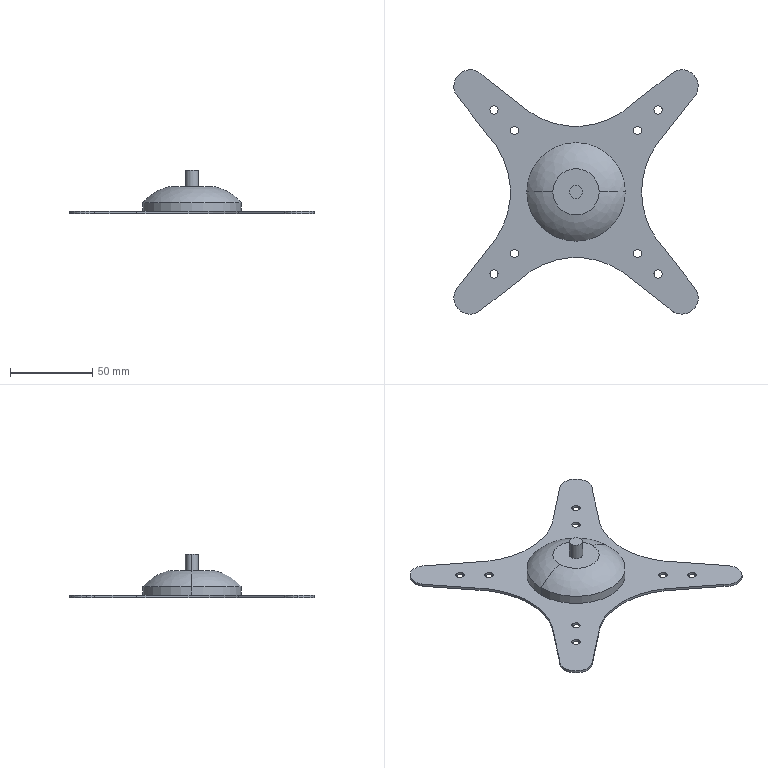Part | SolidWorks | features ICE 3, Extrusion 1, RefAxis 1, RevCut 1 | 1 solid | 45 faces | box 148.985 x 148.985 x 26.5 mm | volume 50583 mm3 | cylinder 31 | plane 12 | spline 2 | commonest cylinder face diameters 5 x16 20 x6 100 x5 8 x2 60 x2
STEP:
#1=CARTESIAN_POINT('',(-30.,0.,6.799));
#2=VERTEX_POINT('',#1);
#3=CARTESIAN_POINT('',(30.,0.,6.799));
#4=VERTEX_POINT('',#3);
#5=CARTESIAN_POINT('',(0.,0.,6.799));
#6=DIRECTION('',(0.,0.,-1.));
#7=DIRECTION('',(-1.,0.,0.));
#8=AXIS2_PLACEMENT_3D('',#5,#6,#7);
#9=CIRCLE('',#8,30.);
#10=EDGE_CURVE('',#2,#4,#9,.T.);
#11=ORIENTED_EDGE('',*,*,#10,.F.);
#12=CARTESIAN_POINT('',(-14.118,0.,16.5));
#13=VERTEX_POINT('',#12);
#14=CARTESIAN_POINT('',(-30.,0.,6.799));
#15=CARTESIAN_POINT('',(-23.65,0.,14.105));
#16=CARTESIAN_POINT('',(-14.118,0.,16.5));
#17=B_SPLINE_CURVE_WITH_KNOTS('',2,(#14,#15,#16),.UNSPECIFIED.,.F.,.F.,(3,3),(0.,1.),.UNSPECIFIED.);
#18=EDGE_CURVE('',#2,#13,#17,.T.);
#19=ORIENTED_EDGE('',*,*,#18,.T.);
#20=CARTESIAN_POINT('',(14.118,0.,16.5));
#21=VERTEX_POINT('',#20);
#22=CARTESIAN_POINT('',(0.,0.,16.5));
#23=DIRECTION('',(0.,0.,-1.));
#24=DIRECTION('',(-1.,0.,0.));
#25=AXIS2_PLACEMENT_3D('',#22,#23,#24);
#26=CIRCLE('',#25,14.118);
#27=EDGE_CURVE('',#13,#21,#26,.T.);
#28=ORIENTED_EDGE('',*,*,#27,.T.);
#29=CARTESIAN_POINT('',(30.,0.,6.799));
#30=CARTESIAN_POINT('',(23.65,0.,14.105));
#31=CARTESIAN_POINT('',(14.118,0.,16.5));
#32=B_SPLINE_CURVE_WITH_KNOTS('',2,(#29,#30,#31),.UNSPECIFIED.,.F.,.F.,(3,3),(0.,1.),.UNSPECIFIED.);
#33=EDGE_CURVE('',#4,#21,#32,.T.);
#34=ORIENTED_EDGE('',*,*,#33,.F.);
#35=EDGE_LOOP('',(#11,#19,#28,#34));
#36=FACE_OUTER_BOUND('',#35,.T.);
#37=CARTESIAN_POINT('',(-30.,0.,6.799));
#38=CARTESIAN_POINT('',(-30.,60.,6.799));
#39=CARTESIAN_POINT('',(30.,60.,6.799));
#40=CARTESIAN_POINT('',(30.,0.,6.799));
#41=CARTESIAN_POINT('',(-23.65,0.,14.105));
#42=CARTESIAN_POINT('',(-23.65,47.299,14.105));
#43=CARTESIAN_POINT('',(23.65,47.299,14.105));
#44=CARTESIAN_POINT('',(23.65,0.,14.105));
#45=CARTESIAN_POINT('',(-14.118,0.,16.5));
#46=CARTESIAN_POINT('',(-14.118,28.237,16.5));
#47=CARTESIAN_POINT('',(14.118,28.237,16.5));
#48=CARTESIAN_POINT('',(14.118,0.,16.5));
#49=(BOUNDED_SURFACE()B_SPLINE_SURFACE(2,3,((#37,#38,#39,#40),(#41,#42,#43,#44),(#45,#46,#47,#48)),.UNSPECIFIED.,.F.,.F.,.F.)B_SPLINE_SURFACE_WITH_KNOTS((3,3),(4,4),(0.,1.),(0.,1.),.UNSPECIFIED.)GEOMETRIC_REPRESENTATION_ITEM()RATIONAL_B_SPLINE_SURFACE(((1.,0.3333,0.3333,1.),(1.,0.3333,0.3333,1.),(1.,0.3333,0.3333,1.)))REPRESENTATION_ITEM('')SURFACE());
#50=ADVANCED_FACE('',(#36),#49,.T.);
#51=CARTESIAN_POINT('',(4.,0.,26.5));
#52=VERTEX_POINT('',#51);
#53=CARTESIAN_POINT('',(-4.,0.,26.5));
#54=VERTEX_POINT('',#53);
#55=CARTESIAN_POINT('',(0.,0.,26.5));
#56=DIRECTION('',(0.,0.,1.));
#57=DIRECTION('',(1.,0.,0.));
#58=AXIS2_PLACEMENT_3D('',#55,#56,#57);
#59=CIRCLE('',#58,4.);
#60=EDGE_CURVE('',#52,#54,#59,.T.);
#61=ORIENTED_EDGE('',*,*,#60,.F.);
#62=CARTESIAN_POINT('',(4.,0.,16.5));
#63=VERTEX_POINT('',#62);
#64=CARTESIAN_POINT('',(4.,0.,26.5));
#65=DIRECTION('',(0.,0.,-1.));
#66=VECTOR('',#65,1000.);
#67=LINE('',#64,#66);
#68=EDGE_CURVE('',#52,#63,#67,.T.);
#69=ORIENTED_EDGE('',*,*,#68,.T.);
#70=CARTESIAN_POINT('',(-4.,0.,16.5));
#71=VERTEX_POINT('',#70);
#72=CARTESIAN_POINT('',(0.,0.,16.5));
#73=DIRECTION('',(0.,0.,1.));
#74=DIRECTION('',(1.,0.,0.));
#75=AXIS2_PLACEMENT_3D('',#72,#73,#74);
#76=CIRCLE('',#75,4.);
#77=EDGE_CURVE('',#63,#71,#76,.T.);
#78=ORIENTED_EDGE('',*,*,#77,.T.);
#79=CARTESIAN_POINT('',(-4.,0.,26.5));
#80=DIRECTION('',(0.,0.,-1.));
#81=VECTOR('',#80,1000.);
#82=LINE('',#79,#81);
#83=EDGE_CURVE('',#54,#71,#82,.T.);
#84=ORIENTED_EDGE('',*,*,#83,.F.);
#85=EDGE_LOOP('',(#61,#69,#78,#84));
#86=FACE_OUTER_BOUND('',#85,.T.);
#87=CARTESIAN_POINT('',(0.,0.,26.5));
#88=DIRECTION('',(0.,0.,-1.));
#89=DIRECTION('',(-1.,0.,0.));
#90=AXIS2_PLACEMENT_3D('',#87,#88,#89);
#91=CYLINDRICAL_SURFACE('',#90,4.);
#92=ADVANCED_FACE('',(#86),#91,.T.);
#93=CARTESIAN_POINT('',(-40.,-37.5,0.));
#94=VERTEX_POINT('',#93);
#95=CARTESIAN_POINT('',(-35.,-37.5,0.));
#96=VERTEX_POINT('',#95);
#97=CARTESIAN_POINT('',(-37.5,-37.5,0.));
#98=DIRECTION('',(0.,0.,1.));
#99=DIRECTION('',(1.,0.,0.));
#100=AXIS2_PLACEMENT_3D('',#97,#98,#99);
#101=CIRCLE('',#100,2.5);
#102=EDGE_CURVE('',#94,#96,#101,.T.);
#103=ORIENTED_EDGE('',*,*,#102,.F.);
#104=CARTESIAN_POINT('',(-40.,-37.5,1.5));
#105=VERTEX_POINT('',#104);
#106=CARTESIAN_POINT('',(-40.,-37.5,0.));
#107=DIRECTION('',(0.,0.,1.));
#108=VECTOR('',#107,1000.);
#109=LINE('',#106,#108);
#110=EDGE_CURVE('',#94,#105,#109,.T.);
#111=ORIENTED_EDGE('',*,*,#110,.T.);
#112=CARTESIAN_POINT('',(-35.,-37.5,1.5));
#113=VERTEX_POINT('',#112);
#114=CARTESIAN_POINT('',(-37.5,-37.5,1.5));
#115=DIRECTION('',(0.,0.,1.));
#116=DIRECTION('',(1.,0.,0.));
#117=AXIS2_PLACEMENT_3D('',#114,#115,#116);
#118=CIRCLE('',#117,2.5);
#119=EDGE_CURVE('',#105,#113,#118,.T.);
#120=ORIENTED_EDGE('',*,*,#119,.T.);
#121=CARTESIAN_POINT('',(-35.,-37.5,0.));
#122=DIRECTION('',(0.,0.,1.));
#123=VECTOR('',#122,1000.);
#124=LINE('',#121,#123);
#125=EDGE_CURVE('',#96,#113,#124,.T.);
#126=ORIENTED_EDGE('',*,*,#125,.F.);
#127=EDGE_LOOP('',(#103,#111,#120,#126));
#128=FACE_OUTER_BOUND('',#127,.T.);
#129=CARTESIAN_POINT('',(-37.5,-37.5,0.));
#130=DIRECTION('',(0.,0.,1.));
#131=DIRECTION('',(1.,0.,0.));
#132=AXIS2_PLACEMENT_3D('',#129,#130,#131);
#133=CYLINDRICAL_SURFACE('',#132,2.5);
#134=ADVANCED_FACE('',(#128),#133,.F.);
#135=CARTESIAN_POINT('',(-52.5,-50.,0.));
#136=VERTEX_POINT('',#135);
#137=CARTESIAN_POINT('',(-47.5,-50.,0.));
#138=VERTEX_POINT('',#137);
#139=CARTESIAN_POINT('',(-50.,-50.,0.));
#140=DIRECTION('',(0.,0.,1.));
#141=DIRECTION('',(1.,0.,0.));
#142=AXIS2_PLACEMENT_3D('',#139,#140,#141);
#143=CIRCLE('',#142,2.5);
#144=EDGE_CURVE('',#136,#138,#143,.T.);
#145=ORIENTED_EDGE('',*,*,#144,.F.);
#146=CARTESIAN_POINT('',(-52.5,-50.,1.5));
#147=VERTEX_POINT('',#146);
#148=CARTESIAN_POINT('',(-52.5,-50.,0.));
#149=DIRECTION('',(0.,0.,1.));
#150=VECTOR('',#149,1000.);
#151=LINE('',#148,#150);
#152=EDGE_CURVE('',#136,#147,#151,.T.);
#153=ORIENTED_EDGE('',*,*,#152,.T.);
#154=CARTESIAN_POINT('',(-47.5,-50.,1.5));
#155=VERTEX_POINT('',#154);
#156=CARTESIAN_POINT('',(-50.,-50.,1.5));
#157=DIRECTION('',(0.,0.,1.));
#158=DIRECTION('',(1.,0.,0.));
#159=AXIS2_PLACEMENT_3D('',#156,#157,#158);
#160=CIRCLE('',#159,2.5);
#161=EDGE_CURVE('',#147,#155,#160,.T.);
#162=ORIENTED_EDGE('',*,*,#161,.T.);
#163=CARTESIAN_POINT('',(-47.5,-50.,0.));
#164=DIRECTION('',(0.,0.,1.));
#165=VECTOR('',#164,1000.);
#166=LINE('',#163,#165);
#167=EDGE_CURVE('',#138,#155,#166,.T.);
#168=ORIENTED_EDGE('',*,*,#167,.F.);
#169=EDGE_LOOP('',(#145,#153,#162,#168));
#170=FACE_OUTER_BOUND('',#169,.T.);
#171=CARTESIAN_POINT('',(-50.,-50.,0.));
#172=DIRECTION('',(0.,0.,1.));
#173=DIRECTION('',(1.,0.,0.));
#174=AXIS2_PLACEMENT_3D('',#171,#172,#173);
#175=CYLINDRICAL_SURFACE('',#174,2.5);
#176=ADVANCED_FACE('',(#170),#175,.F.);
#177=CARTESIAN_POINT('',(35.,-37.5,0.));
#178=VERTEX_POINT('',#177);
#179=CARTESIAN_POINT('',(40.,-37.5,0.));
#180=VERTEX_POINT('',#179);
#181=CARTESIAN_POINT('',(37.5,-37.5,0.));
#182=DIRECTION('',(0.,0.,1.));
#183=DIRECTION('',(1.,0.,0.));
#184=AXIS2_PLACEMENT_3D('',#181,#182,#183);
#185=CIRCLE('',#184,2.5);
#186=EDGE_CURVE('',#178,#180,#185,.T.);
#187=ORIENTED_EDGE('',*,*,#186,.F.);
#188=CARTESIAN_POINT('',(35.,-37.5,1.5));
#189=VERTEX_POINT('',#188);
#190=CARTESIAN_POINT('',(35.,-37.5,0.));
#191=DIRECTION('',(0.,0.,1.));
#192=VECTOR('',#191,1000.);
#193=LINE('',#190,#192);
#194=EDGE_CURVE('',#178,#189,#193,.T.);
#195=ORIENTED_EDGE('',*,*,#194,.T.);
#196=CARTESIAN_POINT('',(40.,-37.5,1.5));
#197=VERTEX_POINT('',#196);
#198=CARTESIAN_POINT('',(37.5,-37.5,1.5));
#199=DIRECTION('',(0.,0.,1.));
#200=DIRECTION('',(1.,0.,0.));
#201=AXIS2_PLACEMENT_3D('',#198,#199,#200);
#202=CIRCLE('',#201,2.5);
#203=EDGE_CURVE('',#189,#197,#202,.T.);
#204=ORIENTED_EDGE('',*,*,#203,.T.);
#205=CARTESIAN_POINT('',(40.,-37.5,0.));
#206=DIRECTION('',(0.,0.,1.));
#207=VECTOR('',#206,1000.);
#208=LINE('',#205,#207);
#209=EDGE_CURVE('',#180,#197,#208,.T.);
#210=ORIENTED_EDGE('',*,*,#209,.F.);
#211=EDGE_LOOP('',(#187,#195,#204,#210));
#212=FACE_OUTER_BOUND('',#211,.T.);
#213=CARTESIAN_POINT('',(37.5,-37.5,0.));
#214=DIRECTION('',(0.,0.,1.));
#215=DIRECTION('',(1.,0.,0.));
#216=AXIS2_PLACEMENT_3D('',#213,#214,#215);
#217=CYLINDRICAL_SURFACE('',#216,2.5);
#218=ADVANCED_FACE('',(#212),#217,.F.);
#219=CARTESIAN_POINT('',(47.5,-50.,0.));
#220=VERTEX_POINT('',#219);
#221=CARTESIAN_POINT('',(52.5,-50.,0.));
#222=VERTEX_POINT('',#221);
#223=CARTESIAN_POINT('',(50.,-50.,0.));
#224=DIRECTION('',(0.,0.,1.));
#225=DIRECTION('',(1.,0.,0.));
#226=AXIS2_PLACEMENT_3D('',#223,#224,#225);
#227=CIRCLE('',#226,2.5);
#228=EDGE_CURVE('',#220,#222,#227,.T.);
#229=ORIENTED_EDGE('',*,*,#228,.F.);
#230=CARTESIAN_POINT('',(47.5,-50.,1.5));
#231=VERTEX_POINT('',#230);
#232=CARTESIAN_POINT('',(47.5,-50.,0.));
#233=DIRECTION('',(0.,0.,1.));
#234=VECTOR('',#233,1000.);
#235=LINE('',#232,#234);
#236=EDGE_CURVE('',#220,#231,#235,.T.);
#237=ORIENTED_EDGE('',*,*,#236,.T.);
#238=CARTESIAN_POINT('',(52.5,-50.,1.5));
#239=VERTEX_POINT('',#238);
#240=CARTESIAN_POINT('',(50.,-50.,1.5));
#241=DIRECTION('',(0.,0.,1.));
#242=DIRECTION('',(1.,0.,0.));
#243=AXIS2_PLACEMENT_3D('',#240,#241,#242);
#244=CIRCLE('',#243,2.5);
#245=EDGE_CURVE('',#231,#239,#244,.T.);
#246=ORIENTED_EDGE('',*,*,#245,.T.);
#247=CARTESIAN_POINT('',(52.5,-50.,0.));
#248=DIRECTION('',(0.,0.,1.));
#249=VECTOR('',#248,1000.);
#250=LINE('',#247,#249);
#251=EDGE_CURVE('',#222,#239,#250,.T.);
#252=ORIENTED_EDGE('',*,*,#251,.F.);
#253=EDGE_LOOP('',(#229,#237,#246,#252));
#254=FACE_OUTER_BOUND('',#253,.T.);
#255=CARTESIAN_POINT('',(50.,-50.,0.));
#256=DIRECTION('',(0.,0.,1.));
#257=DIRECTION('',(1.,0.,0.));
#258=AXIS2_PLACEMENT_3D('',#255,#256,#257);
#259=CYLINDRICAL_SURFACE('',#258,2.5);
#260=ADVANCED_FACE('',(#254),#259,.F.);
#261=CARTESIAN_POINT('',(35.,37.5,0.));
#262=VERTEX_POINT('',#261);
#263=CARTESIAN_POINT('',(40.,37.5,0.));
#264=VERTEX_POINT('',#263);
#265=CARTESIAN_POINT('',(37.5,37.5,0.));
#266=DIRECTION('',(0.,0.,1.));
#267=DIRECTION('',(1.,0.,0.));
#268=AXIS2_PLACEMENT_3D('',#265,#266,#267);
#269=CIRCLE('',#268,2.5);
#270=EDGE_CURVE('',#262,#264,#269,.T.);
#271=ORIENTED_EDGE('',*,*,#270,.F.);
#272=CARTESIAN_POINT('',(35.,37.5,1.5));
#273=VERTEX_POINT('',#272);
#274=CARTESIAN_POINT('',(35.,37.5,0.));
#275=DIRECTION('',(0.,0.,1.));
#276=VECTOR('',#275,1000.);
#277=LINE('',#274,#276);
#278=EDGE_CURVE('',#262,#273,#277,.T.);
#279=ORIENTED_EDGE('',*,*,#278,.T.);
#280=CARTESIAN_POINT('',(40.,37.5,1.5));
#281=VERTEX_POINT('',#280);
#282=CARTESIAN_POINT('',(37.5,37.5,1.5));
#283=DIRECTION('',(0.,0.,1.));
#284=DIRECTION('',(1.,0.,0.));
#285=AXIS2_PLACEMENT_3D('',#282,#283,#284);
#286=CIRCLE('',#285,2.5);
#287=EDGE_CURVE('',#273,#281,#286,.T.);
#288=ORIENTED_EDGE('',*,*,#287,.T.);
#289=CARTESIAN_POINT('',(40.,37.5,0.));
#290=DIRECTION('',(0.,0.,1.));
#291=VECTOR('',#290,1000.);
#292=LINE('',#289,#291);
#293=EDGE_CURVE('',#264,#281,#292,.T.);
#294=ORIENTED_EDGE('',*,*,#293,.F.);
#295=EDGE_LOOP('',(#271,#279,#288,#294));
#296=FACE_OUTER_BOUND('',#295,.T.);
#297=CARTESIAN_POINT('',(37.5,37.5,0.));
#298=DIRECTION('',(0.,0.,1.));
#299=DIRECTION('',(1.,0.,0.));
#300=AXIS2_PLACEMENT_3D('',#297,#298,#299);
#301=CYLINDRICAL_SURFACE('',#300,2.5);
#302=ADVANCED_FACE('',(#296),#301,.F.);
#303=CARTESIAN_POINT('',(47.5,50.,0.));
#304=VERTEX_POINT('',#303);
#305=CARTESIAN_POINT('',(52.5,50.,0.));
#306=VERTEX_POINT('',#305);
#307=CARTESIAN_POINT('',(50.,50.,0.));
#308=DIRECTION('',(0.,0.,1.));
#309=DIRECTION('',(1.,0.,0.));
#310=AXIS2_PLACEMENT_3D('',#307,#308,#309);
#311=CIRCLE('',#310,2.5);
#312=EDGE_CURVE('',#304,#306,#311,.T.);
#313=ORIENTED_EDGE('',*,*,#312,.F.);
#314=CARTESIAN_POINT('',(47.5,50.,1.5));
#315=VERTEX_POINT('',#314);
#316=CARTESIAN_POINT('',(47.5,50.,0.));
#317=DIRECTION('',(0.,0.,1.));
#318=VECTOR('',#317,1000.);
#319=LINE('',#316,#318);
#320=EDGE_CURVE('',#304,#315,#319,.T.);
#321=ORIENTED_EDGE('',*,*,#320,.T.);
#322=CARTESIAN_POINT('',(52.5,50.,1.5));
#323=VERTEX_POINT('',#322);
#324=CARTESIAN_POINT('',(50.,50.,1.5));
#325=DIRECTION('',(0.,0.,1.));
#326=DIRECTION('',(1.,0.,0.));
#327=AXIS2_PLACEMENT_3D('',#324,#325,#326);
#328=CIRCLE('',#327,2.5);
#329=EDGE_CURVE('',#315,#323,#328,.T.);
#330=ORIENTED_EDGE('',*,*,#329,.T.);
#331=CARTESIAN_POINT('',(52.5,50.,0.));
#332=DIRECTION('',(0.,0.,1.));
#333=VECTOR('',#332,1000.);
#334=LINE('',#331,#333);
#335=EDGE_CURVE('',#306,#323,#334,.T.);
#336=ORIENTED_EDGE('',*,*,#335,.F.);
#337=EDGE_LOOP('',(#313,#321,#330,#336));
#338=FACE_OUTER_BOUND('',#337,.T.);
#339=CARTESIAN_POINT('',(50.,50.,0.));
#340=DIRECTION('',(0.,0.,1.));
#341=DIRECTION('',(1.,0.,0.));
#342=AXIS2_PLACEMENT_3D('',#339,#340,#341);
#343=CYLINDRICAL_SURFACE('',#342,2.5);
#344=ADVANCED_FACE('',(#338),#343,.F.);
#345=CARTESIAN_POINT('',(-40.,37.5,0.));
#346=VERTEX_POINT('',#345);
#347=CARTESIAN_POINT('',(-35.,37.5,0.));
#348=VERTEX_POINT('',#347);
#349=CARTESIAN_POINT('',(-37.5,37.5,0.));
#350=DIRECTION('',(0.,0.,1.));
#351=DIRECTION('',(1.,0.,0.));
#352=AXIS2_PLACEMENT_3D('',#349,#350,#351);
#353=CIRCLE('',#352,2.5);
#354=EDGE_CURVE('',#346,#348,#353,.T.);
#355=ORIENTED_EDGE('',*,*,#354,.F.);
#356=CARTESIAN_POINT('',(-40.,37.5,1.5));
#357=VERTEX_POINT('',#356);
#358=CARTESIAN_POINT('',(-40.,37.5,0.));
#359=DIRECTION('',(0.,0.,1.));
#360=VECTOR('',#359,1000.);
#361=LINE('',#358,#360);
#362=EDGE_CURVE('',#346,#357,#361,.T.);
#363=ORIENTED_EDGE('',*,*,#362,.T.);
#364=CARTESIAN_POINT('',(-35.,37.5,1.5));
#365=VERTEX_POINT('',#364);
#366=CARTESIAN_POINT('',(-37.5,37.5,1.5));
#367=DIRECTION('',(0.,0.,1.));
#368=DIRECTION('',(1.,0.,0.));
#369=AXIS2_PLACEMENT_3D('',#366,#367,#368);
#370=CIRCLE('',#369,2.5);
#371=EDGE_CURVE('',#357,#365,#370,.T.);
#372=ORIENTED_EDGE('',*,*,#371,.T.);
#373=CARTESIAN_POINT('',(-35.,37.5,0.));
#374=DIRECTION('',(0.,0.,1.));
#375=VECTOR('',#374,1000.);
#376=LINE('',#373,#375);
#377=EDGE_CURVE('',#348,#365,#376,.T.);
#378=ORIENTED_EDGE('',*,*,#377,.F.);
#379=EDGE_LOOP('',(#355,#363,#372,#378));
#380=FACE_OUTER_BOUND('',#379,.T.);
#381=CARTESIAN_POINT('',(-37.5,37.5,0.));
#382=DIRECTION('',(0.,0.,1.));
#383=DIRECTION('',(1.,0.,0.));
#384=AXIS2_PLACEMENT_3D('',#381,#382,#383);
#385=CYLINDRICAL_SURFACE('',#384,2.5);
#386=ADVANCED_FACE('',(#380),#385,.F.);
#387=CARTESIAN_POINT('',(-52.5,50.,0.));
#388=VERTEX_POINT('',#387);
#389=CARTESIAN_POINT('',(-47.5,50.,0.));
#390=VERTEX_POINT('',#389);
#391=CARTESIAN_POINT('',(-50.,50.,0.));
#392=DIRECTION('',(0.,0.,1.));
#393=DIRECTION('',(1.,0.,0.));
#394=AXIS2_PLACEMENT_3D('',#391,#392,#393);
#395=CIRCLE('',#394,2.5);
#396=EDGE_CURVE('',#388,#390,#395,.T.);
#397=ORIENTED_EDGE('',*,*,#396,.F.);
#398=CARTESIAN_POINT('',(-52.5,50.,1.5));
#399=VERTEX_POINT('',#398);
#400=CARTESIAN_POINT('',(-52.5,50.,0.));
#401=DIRECTION('',(0.,0.,1.));
#402=VECTOR('',#401,1000.);
#403=LINE('',#400,#402);
#404=EDGE_CURVE('',#388,#399,#403,.T.);
#405=ORIENTED_EDGE('',*,*,#404,.T.);
#406=CARTESIAN_POINT('',(-47.5,50.,1.5));
#407=VERTEX_POINT('',#406);
#408=CARTESIAN_POINT('',(-50.,50.,1.5));
#409=DIRECTION('',(0.,0.,1.));
#410=DIRECTION('',(1.,0.,0.));
#411=AXIS2_PLACEMENT_3D('',#408,#409,#410);
#412=CIRCLE('',#411,2.5);
#413=EDGE_CURVE('',#399,#407,#412,.T.);
#414=ORIENTED_EDGE('',*,*,#413,.T.);
#415=CARTESIAN_POINT('',(-47.5,50.,0.));
#416=DIRECTION('',(0.,0.,1.));
#417=VECTOR('',#416,1000.);
#418=LINE('',#415,#417);
#419=EDGE_CURVE('',#390,#407,#418,.T.);
#420=ORIENTED_EDGE('',*,*,#419,.F.);
#421=EDGE_LOOP('',(#397,#405,#414,#420));
#422=FACE_OUTER_BOUND('',#421,.T.);
#423=CARTESIAN_POINT('',(-50.,50.,0.));
#424=DIRECTION('',(0.,0.,1.));
#425=DIRECTION('',(1.,0.,0.));
#426=AXIS2_PLACEMENT_3D('',#423,#424,#425);
#427=CYLINDRICAL_SURFACE('',#426,2.5);
#428=ADVANCED_FACE('',(#422),#427,.F.);
#429=CARTESIAN_POINT('',(-74.493,64.493,1.5));
#430=VERTEX_POINT('',#429);
#431=CARTESIAN_POINT('',(-72.99,59.22,1.5));
#432=VERTEX_POINT('',#431);
#433=CARTESIAN_POINT('',(-64.493,64.493,1.5));
#434=DIRECTION('',(0.,0.,1.));
#435=DIRECTION('',(1.,0.,0.));
#436=AXIS2_PLACEMENT_3D('',#433,#434,#435);
#437=CIRCLE('',#436,10.);
#438=EDGE_CURVE('',#430,#432,#437,.T.);
#439=ORIENTED_EDGE('',*,*,#438,.F.);
#440=CARTESIAN_POINT('',(-74.493,64.493,0.));
#441=VERTEX_POINT('',#440);
#442=CARTESIAN_POINT('',(-74.493,64.493,1.5));
#443=DIRECTION('',(0.,0.,-1.));
#444=VECTOR('',#443,1000.);
#445=LINE('',#442,#444);
#446=EDGE_CURVE('',#430,#441,#445,.T.);
#447=ORIENTED_EDGE('',*,*,#446,.T.);
#448=CARTESIAN_POINT('',(-72.99,59.22,0.));
#449=VERTEX_POINT('',#448);
#450=CARTESIAN_POINT('',(-64.493,64.493,0.));
#451=DIRECTION('',(0.,0.,1.));
#452=DIRECTION('',(1.,0.,0.));
#453=AXIS2_PLACEMENT_3D('',#450,#451,#452);
#454=CIRCLE('',#453,10.);
#455=EDGE_CURVE('',#441,#449,#454,.T.);
#456=ORIENTED_EDGE('',*,*,#455,.T.);
#457=CARTESIAN_POINT('',(-72.99,59.22,1.5));
#458=DIRECTION('',(0.,0.,-1.));
#459=VECTOR('',#458,1000.);
#460=LINE('',#457,#459);
#461=EDGE_CURVE('',#432,#449,#460,.T.);
#462=ORIENTED_EDGE('',*,*,#461,.F.);
#463=EDGE_LOOP('',(#439,#447,#456,#462));
#464=FACE_OUTER_BOUND('',#463,.T.);
#465=CARTESIAN_POINT('',(-64.493,64.493,1.5));
#466=DIRECTION('',(0.,0.,-1.));
#467=DIRECTION('',(-1.,0.,0.));
#468=AXIS2_PLACEMENT_3D('',#465,#466,#467);
#469=CYLINDRICAL_SURFACE('',#468,10.);
#470=ADVANCED_FACE('',(#464),#469,.T.);
#471=CARTESIAN_POINT('',(40.,0.,1.5));
#472=VERTEX_POINT('',#471);
#473=CARTESIAN_POINT('',(48.656,28.119,1.5));
#474=VERTEX_POINT('',#473);
#475=CARTESIAN_POINT('',(90.,0.,1.5));
#476=DIRECTION('',(0.,0.,-1.));
#477=DIRECTION('',(1.,0.,0.));
#478=AXIS2_PLACEMENT_3D('',#475,#476,#477);
#479=CIRCLE('',#478,50.);
#480=EDGE_CURVE('',#472,#474,#479,.T.);
#481=ORIENTED_EDGE('',*,*,#480,.F.);
#482=CARTESIAN_POINT('',(40.,0.,0.));
#483=VERTEX_POINT('',#482);
#484=CARTESIAN_POINT('',(40.,0.,1.5));
#485=DIRECTION('',(0.,0.,-1.));
#486=VECTOR('',#485,1000.);
#487=LINE('',#484,#486);
#488=EDGE_CURVE('',#472,#483,#487,.T.);
#489=ORIENTED_EDGE('',*,*,#488,.T.);
#490=CARTESIAN_POINT('',(48.656,28.119,0.));
#491=VERTEX_POINT('',#490);
#492=CARTESIAN_POINT('',(90.,0.,0.));
#493=DIRECTION('',(0.,0.,-1.));
#494=DIRECTION('',(1.,0.,0.));
#495=AXIS2_PLACEMENT_3D('',#492,#493,#494);
#496=CIRCLE('',#495,50.);
#497=EDGE_CURVE('',#483,#491,#496,.T.);
#498=ORIENTED_EDGE('',*,*,#497,.T.);
#499=CARTESIAN_POINT('',(48.656,28.119,1.5));
#500=DIRECTION('',(0.,0.,-1.));
#501=VECTOR('',#500,1000.);
#502=LINE('',#499,#501);
#503=EDGE_CURVE('',#474,#491,#502,.T.);
#504=ORIENTED_EDGE('',*,*,#503,.F.);
#505=EDGE_LOOP('',(#481,#489,#498,#504));
#506=FACE_OUTER_BOUND('',#505,.T.);
#507=CARTESIAN_POINT('',(90.,0.,1.5));
#508=DIRECTION('',(0.,0.,-1.));
#509=DIRECTION('',(-1.,0.,0.));
#510=AXIS2_PLACEMENT_3D('',#507,#508,#509);
#511=CYLINDRICAL_SURFACE('',#510,50.);
#512=ADVANCED_FACE('',(#506),#511,.F.);
#513=CARTESIAN_POINT('',(-74.493,-64.493,1.5));
#514=VERTEX_POINT('',#513);
#515=CARTESIAN_POINT('',(-59.22,-72.99,1.5));
#516=VERTEX_POINT('',#515);
#517=CARTESIAN_POINT('',(-64.493,-64.493,1.5));
#518=DIRECTION('',(0.,0.,1.));
#519=DIRECTION('',(1.,0.,0.));
#520=AXIS2_PLACEMENT_3D('',#517,#518,#519);
#521=CIRCLE('',#520,10.);
#522=EDGE_CURVE('',#514,#516,#521,.T.);
#523=ORIENTED_EDGE('',*,*,#522,.F.);
#524=CARTESIAN_POINT('',(-74.493,-64.493,0.));
#525=VERTEX_POINT('',#524);
#526=CARTESIAN_POINT('',(-74.493,-64.493,1.5));
#527=DIRECTION('',(0.,0.,-1.));
#528=VECTOR('',#527,1000.);
#529=LINE('',#526,#528);
#530=EDGE_CURVE('',#514,#525,#529,.T.);
#531=ORIENTED_EDGE('',*,*,#530,.T.);
#532=CARTESIAN_POINT('',(-59.22,-72.99,0.));
#533=VERTEX_POINT('',#532);
#534=CARTESIAN_POINT('',(-64.493,-64.493,0.));
#535=DIRECTION('',(0.,0.,1.));
#536=DIRECTION('',(1.,0.,0.));
#537=AXIS2_PLACEMENT_3D('',#534,#535,#536);
#538=CIRCLE('',#537,10.);
#539=EDGE_CURVE('',#525,#533,#538,.T.);
#540=ORIENTED_EDGE('',*,*,#539,.T.);
#541=CARTESIAN_POINT('',(-59.22,-72.99,1.5));
#542=DIRECTION('',(0.,0.,-1.));
#543=VECTOR('',#542,1000.);
#544=LINE('',#541,#543);
#545=EDGE_CURVE('',#516,#533,#544,.T.);
#546=ORIENTED_EDGE('',*,*,#545,.F.);
#547=EDGE_LOOP('',(#523,#531,#540,#546));
#548=FACE_OUTER_BOUND('',#547,.T.);
#549=CARTESIAN_POINT('',(-64.493,-64.493,1.5));
#550=DIRECTION('',(0.,0.,-1.));
#551=DIRECTION('',(-1.,0.,0.));
#552=AXIS2_PLACEMENT_3D('',#549,#550,#551);
#553=CYLINDRICAL_SURFACE('',#552,10.);
#554=ADVANCED_FACE('',(#548),#553,.T.);
#555=ORIENTED_EDGE('',*,*,#10,.T.);
#556=CARTESIAN_POINT('',(30.,0.,1.5));
#557=VERTEX_POINT('',#556);
#558=CARTESIAN_POINT('',(30.,0.,16.5));
#559=DIRECTION('',(0.,0.,-1.));
#560=VECTOR('',#559,1000.);
#561=LINE('',#558,#560);
#562=EDGE_CURVE('',#4,#557,#561,.T.);
#563=ORIENTED_EDGE('',*,*,#562,.T.);
#564=CARTESIAN_POINT('',(-30.,0.,1.5));
#565=VERTEX_POINT('',#564);
#566=CARTESIAN_POINT('',(0.,0.,1.5));
#567=DIRECTION('',(0.,0.,1.));
#568=DIRECTION('',(1.,0.,0.));
#569=AXIS2_PLACEMENT_3D('',#566,#567,#568);
#570=CIRCLE('',#569,30.);
#571=EDGE_CURVE('',#557,#565,#570,.T.);
#572=ORIENTED_EDGE('',*,*,#571,.T.);
#573=CARTESIAN_POINT('',(-30.,0.,16.5));
#574=DIRECTION('',(0.,0.,-1.));
#575=VECTOR('',#574,1000.);
#576=LINE('',#573,#575);
#577=EDGE_CURVE('',#2,#565,#576,.T.);
#578=ORIENTED_EDGE('',*,*,#577,.F.);
#579=EDGE_LOOP('',(#555,#563,#572,#578));
#580=FACE_OUTER_BOUND('',#579,.T.);
#581=CARTESIAN_POINT('',(0.,0.,16.5));
#582=DIRECTION('',(0.,0.,-1.));
#583=DIRECTION('',(-1.,0.,0.));
#584=AXIS2_PLACEMENT_3D('',#581,#582,#583);
#585=CYLINDRICAL_SURFACE('',#584,30.);
#586=ADVANCED_FACE('',(#580),#585,.T.);
#587=CARTESIAN_POINT('',(0.,0.,16.5));
#588=DIRECTION('',(0.,0.,-1.));
#589=DIRECTION('',(-1.,0.,0.));
#590=AXIS2_PLACEMENT_3D('',#587,#588,#589);
#591=CIRCLE('',#590,14.118);
#592=EDGE_CURVE('',#21,#13,#591,.T.);
#593=ORIENTED_EDGE('',*,*,#592,.F.);
#594=ORIENTED_EDGE('',*,*,#27,.F.);
#595=EDGE_LOOP('',(#593,#594));
#596=FACE_OUTER_BOUND('',#595,.T.);
#597=CARTESIAN_POINT('',(0.,0.,16.5));
#598=DIRECTION('',(0.,0.,1.));
#599=DIRECTION('',(1.,0.,0.));
#600=AXIS2_PLACEMENT_3D('',#597,#598,#599);
#601=CIRCLE('',#600,4.);
#602=EDGE_CURVE('',#71,#63,#601,.T.);
#603=ORIENTED_EDGE('',*,*,#602,.F.);
#604=ORIENTED_EDGE('',*,*,#77,.F.);
#605=EDGE_LOOP('',(#603,#604));
#606=FACE_BOUND('',#605,.T.);
#607=CARTESIAN_POINT('',(0.,0.,16.5));
#608=DIRECTION('',(0.,0.,1.));
#609=DIRECTION('',(1.,0.,0.));
#610=AXIS2_PLACEMENT_3D('',#607,#608,#609);
#611=PLANE('',#610);
#612=ADVANCED_FACE('',(#596,#606),#611,.T.);
#613=ORIENTED_EDGE('',*,*,#562,.F.);
#614=CARTESIAN_POINT('',(0.,0.,6.799));
#615=DIRECTION('',(0.,0.,-1.));
#616=DIRECTION('',(-1.,0.,0.));
#617=AXIS2_PLACEMENT_3D('',#614,#615,#616);
#618=CIRCLE('',#617,30.);
#619=EDGE_CURVE('',#4,#2,#618,.T.);
#620=ORIENTED_EDGE('',*,*,#619,.T.);
#621=ORIENTED_EDGE('',*,*,#577,.T.);
#622=CARTESIAN_POINT('',(0.,0.,1.5));
#623=DIRECTION('',(0.,0.,1.));
#624=DIRECTION('',(1.,0.,0.));
#625=AXIS2_PLACEMENT_3D('',#622,#623,#624);
#626=CIRCLE('',#625,30.);
#627=EDGE_CURVE('',#565,#557,#626,.T.);
#628=ORIENTED_EDGE('',*,*,#627,.T.);
#629=EDGE_LOOP('',(#613,#620,#621,#628));
#630=FACE_OUTER_BOUND('',#629,.T.);
#631=CARTESIAN_POINT('',(0.,0.,16.5));
#632=DIRECTION('',(0.,0.,-1.));
#633=DIRECTION('',(-1.,0.,0.));
#634=AXIS2_PLACEMENT_3D('',#631,#632,#633);
#635=CYLINDRICAL_SURFACE('',#634,30.);
#636=ADVANCED_FACE('',(#630),#635,.T.);
#637=CARTESIAN_POINT('',(-53.317,33.976,1.5));
#638=VERTEX_POINT('',#637);
#639=CARTESIAN_POINT('',(-72.99,59.22,1.5));
#640=CARTESIAN_POINT('',(-53.317,33.976,1.5));
#641=B_SPLINE_CURVE_WITH_KNOTS('',1,(#639,#640),.UNSPECIFIED.,.F.,.F.,(2,2),(0.,1.),.UNSPECIFIED.);
#642=EDGE_CURVE('',#432,#638,#641,.T.);
#643=ORIENTED_EDGE('',*,*,#642,.T.);
#644=CARTESIAN_POINT('',(-48.656,-28.119,1.5));
#645=VERTEX_POINT('',#644);
#646=CARTESIAN_POINT('',(-90.,0.,1.5));
#647=DIRECTION('',(0.,0.,-1.));
#648=DIRECTION('',(1.,0.,0.));
#649=AXIS2_PLACEMENT_3D('',#646,#647,#648);
#650=CIRCLE('',#649,50.);
#651=EDGE_CURVE('',#638,#645,#650,.T.);
#652=ORIENTED_EDGE('',*,*,#651,.T.);
#653=CARTESIAN_POINT('',(-70.727,-56.674,1.5));
#654=VERTEX_POINT('',#653);
#655=CARTESIAN_POINT('',(-48.656,-28.119,1.5));
#656=CARTESIAN_POINT('',(-70.727,-56.674,1.5));
#657=B_SPLINE_CURVE_WITH_KNOTS('',1,(#655,#656),.UNSPECIFIED.,.F.,.F.,(2,2),(0.,1.),.UNSPECIFIED.);
#658=EDGE_CURVE('',#645,#654,#657,.T.);
#659=ORIENTED_EDGE('',*,*,#658,.T.);
#660=CARTESIAN_POINT('',(-64.493,-64.493,1.5));
#661=DIRECTION('',(0.,0.,1.));
#662=DIRECTION('',(1.,0.,0.));
#663=AXIS2_PLACEMENT_3D('',#660,#661,#662);
#664=CIRCLE('',#663,10.);
#665=EDGE_CURVE('',#654,#514,#664,.T.);
#666=ORIENTED_EDGE('',*,*,#665,.T.);
#667=ORIENTED_EDGE('',*,*,#522,.T.);
#668=CARTESIAN_POINT('',(-33.976,-53.317,1.5));
#669=VERTEX_POINT('',#668);
#670=CARTESIAN_POINT('',(-59.22,-72.99,1.5));
#671=CARTESIAN_POINT('',(-33.976,-53.317,1.5));
#672=B_SPLINE_CURVE_WITH_KNOTS('',1,(#670,#671),.UNSPECIFIED.,.F.,.F.,(2,2),(0.,1.),.UNSPECIFIED.);
#673=EDGE_CURVE('',#516,#669,#672,.T.);
#674=ORIENTED_EDGE('',*,*,#673,.T.);
#675=CARTESIAN_POINT('',(28.119,-48.656,1.5));
#676=VERTEX_POINT('',#675);
#677=CARTESIAN_POINT('',(0.,-90.,1.5));
#678=DIRECTION('',(0.,0.,-1.));
#679=DIRECTION('',(1.,0.,0.));
#680=AXIS2_PLACEMENT_3D('',#677,#678,#679);
#681=CIRCLE('',#680,50.);
#682=EDGE_CURVE('',#669,#676,#681,.T.);
#683=ORIENTED_EDGE('',*,*,#682,.T.);
#684=CARTESIAN_POINT('',(56.674,-70.727,1.5));
#685=VERTEX_POINT('',#684);
#686=CARTESIAN_POINT('',(28.119,-48.656,1.5));
#687=CARTESIAN_POINT('',(56.674,-70.727,1.5));
#688=B_SPLINE_CURVE_WITH_KNOTS('',1,(#686,#687),.UNSPECIFIED.,.F.,.F.,(2,2),(0.,1.),.UNSPECIFIED.);
#689=EDGE_CURVE('',#676,#685,#688,.T.);
#690=ORIENTED_EDGE('',*,*,#689,.T.);
#691=CARTESIAN_POINT('',(72.99,-59.22,1.5));
#692=VERTEX_POINT('',#691);
#693=CARTESIAN_POINT('',(64.493,-64.493,1.5));
#694=DIRECTION('',(0.,0.,1.));
#695=DIRECTION('',(1.,0.,0.));
#696=AXIS2_PLACEMENT_3D('',#693,#694,#695);
#697=CIRCLE('',#696,10.);
#698=EDGE_CURVE('',#685,#692,#697,.T.);
#699=ORIENTED_EDGE('',*,*,#698,.T.);
#700=CARTESIAN_POINT('',(53.317,-33.976,1.5));
#701=VERTEX_POINT('',#700);
#702=CARTESIAN_POINT('',(72.99,-59.22,1.5));
#703=CARTESIAN_POINT('',(53.317,-33.976,1.5));
#704=B_SPLINE_CURVE_WITH_KNOTS('',1,(#702,#703),.UNSPECIFIED.,.F.,.F.,(2,2),(0.,1.),.UNSPECIFIED.);
#705=EDGE_CURVE('',#692,#701,#704,.T.);
#706=ORIENTED_EDGE('',*,*,#705,.T.);
#707=CARTESIAN_POINT('',(90.,0.,1.5));
#708=DIRECTION('',(0.,0.,-1.));
#709=DIRECTION('',(1.,0.,0.));
#710=AXIS2_PLACEMENT_3D('',#707,#708,#709);
#711=CIRCLE('',#710,50.);
#712=EDGE_CURVE('',#701,#472,#711,.T.);
#713=ORIENTED_EDGE('',*,*,#712,.T.);
#714=ORIENTED_EDGE('',*,*,#480,.T.);
#715=CARTESIAN_POINT('',(70.727,56.674,1.5));
#716=VERTEX_POINT('',#715);
#717=CARTESIAN_POINT('',(48.656,28.119,1.5));
#718=CARTESIAN_POINT('',(70.727,56.674,1.5));
#719=B_SPLINE_CURVE_WITH_KNOTS('',1,(#717,#718),.UNSPECIFIED.,.F.,.F.,(2,2),(0.,1.),.UNSPECIFIED.);
#720=EDGE_CURVE('',#474,#716,#719,.T.);
#721=ORIENTED_EDGE('',*,*,#720,.T.);
#722=CARTESIAN_POINT('',(59.22,72.99,1.5));
#723=VERTEX_POINT('',#722);
#724=CARTESIAN_POINT('',(64.493,64.493,1.5));
#725=DIRECTION('',(0.,0.,1.));
#726=DIRECTION('',(1.,0.,0.));
#727=AXIS2_PLACEMENT_3D('',#724,#725,#726);
#728=CIRCLE('',#727,10.);
#729=EDGE_CURVE('',#716,#723,#728,.T.);
#730=ORIENTED_EDGE('',*,*,#729,.T.);
#731=CARTESIAN_POINT('',(33.976,53.317,1.5));
#732=VERTEX_POINT('',#731);
#733=CARTESIAN_POINT('',(59.22,72.99,1.5));
#734=CARTESIAN_POINT('',(33.976,53.317,1.5));
#735=B_SPLINE_CURVE_WITH_KNOTS('',1,(#733,#734),.UNSPECIFIED.,.F.,.F.,(2,2),(0.,1.),.UNSPECIFIED.);
#736=EDGE_CURVE('',#723,#732,#735,.T.);
#737=ORIENTED_EDGE('',*,*,#736,.T.);
#738=CARTESIAN_POINT('',(-28.119,48.656,1.5));
#739=VERTEX_POINT('',#738);
#740=CARTESIAN_POINT('',(0.,90.,1.5));
#741=DIRECTION('',(0.,0.,-1.));
#742=DIRECTION('',(1.,0.,0.));
#743=AXIS2_PLACEMENT_3D('',#740,#741,#742);
#744=CIRCLE('',#743,50.);
#745=EDGE_CURVE('',#732,#739,#744,.T.);
#746=ORIENTED_EDGE('',*,*,#745,.T.);
#747=CARTESIAN_POINT('',(-56.674,70.727,1.5));
#748=VERTEX_POINT('',#747);
#749=CARTESIAN_POINT('',(-28.119,48.656,1.5));
#750=CARTESIAN_POINT('',(-56.674,70.727,1.5));
#751=B_SPLINE_CURVE_WITH_KNOTS('',1,(#749,#750),.UNSPECIFIED.,.F.,.F.,(2,2),(0.,1.),.UNSPECIFIED.);
#752=EDGE_CURVE('',#739,#748,#751,.T.);
#753=ORIENTED_EDGE('',*,*,#752,.T.);
#754=CARTESIAN_POINT('',(-64.493,64.493,1.5));
#755=DIRECTION('',(0.,0.,1.));
#756=DIRECTION('',(1.,0.,0.));
#757=AXIS2_PLACEMENT_3D('',#754,#755,#756);
#758=CIRCLE('',#757,10.);
#759=EDGE_CURVE('',#748,#430,#758,.T.);
#760=ORIENTED_EDGE('',*,*,#759,.T.);
#761=ORIENTED_EDGE('',*,*,#438,.T.);
#762=EDGE_LOOP('',(#643,#652,#659,#666,#667,#674,#683,#690,#699,#706,#713,#714,#721,#730,#737,#746,#753,#760,#761));
#763=FACE_OUTER_BOUND('',#762,.T.);
#764=CARTESIAN_POINT('',(-50.,50.,1.5));
#765=DIRECTION('',(0.,0.,1.));
#766=DIRECTION('',(1.,0.,0.));
#767=AXIS2_PLACEMENT_3D('',#764,#765,#766);
#768=CIRCLE('',#767,2.5);
#769=EDGE_CURVE('',#407,#399,#768,.T.);
#770=ORIENTED_EDGE('',*,*,#769,.F.);
#771=ORIENTED_EDGE('',*,*,#413,.F.);
#772=EDGE_LOOP('',(#770,#771));
#773=FACE_BOUND('',#772,.T.);
#774=CARTESIAN_POINT('',(-37.5,37.5,1.5));
#775=DIRECTION('',(0.,0.,1.));
#776=DIRECTION('',(1.,0.,0.));
#777=AXIS2_PLACEMENT_3D('',#774,#775,#776);
#778=CIRCLE('',#777,2.5);
#779=EDGE_CURVE('',#365,#357,#778,.T.);
#780=ORIENTED_EDGE('',*,*,#779,.F.);
#781=ORIENTED_EDGE('',*,*,#371,.F.);
#782=EDGE_LOOP('',(#780,#781));
#783=FACE_BOUND('',#782,.T.);
#784=CARTESIAN_POINT('',(50.,50.,1.5));
#785=DIRECTION('',(0.,0.,1.));
#786=DIRECTION('',(1.,0.,0.));
#787=AXIS2_PLACEMENT_3D('',#784,#785,#786);
#788=CIRCLE('',#787,2.5);
#789=EDGE_CURVE('',#323,#315,#788,.T.);
#790=ORIENTED_EDGE('',*,*,#789,.F.);
#791=ORIENTED_EDGE('',*,*,#329,.F.);
#792=EDGE_LOOP('',(#790,#791));
#793=FACE_BOUND('',#792,.T.);
#794=CARTESIAN_POINT('',(37.5,37.5,1.5));
#795=DIRECTION('',(0.,0.,1.));
#796=DIRECTION('',(1.,0.,0.));
#797=AXIS2_PLACEMENT_3D('',#794,#795,#796);
#798=CIRCLE('',#797,2.5);
#799=EDGE_CURVE('',#281,#273,#798,.T.);
#800=ORIENTED_EDGE('',*,*,#799,.F.);
#801=ORIENTED_EDGE('',*,*,#287,.F.);
#802=EDGE_LOOP('',(#800,#801));
#803=FACE_BOUND('',#802,.T.);
#804=CARTESIAN_POINT('',(50.,-50.,1.5));
#805=DIRECTION('',(0.,0.,1.));
#806=DIRECTION('',(1.,0.,0.));
#807=AXIS2_PLACEMENT_3D('',#804,#805,#806);
#808=CIRCLE('',#807,2.5);
#809=EDGE_CURVE('',#239,#231,#808,.T.);
#810=ORIENTED_EDGE('',*,*,#809,.F.);
#811=ORIENTED_EDGE('',*,*,#245,.F.);
#812=EDGE_LOOP('',(#810,#811));
#813=FACE_BOUND('',#812,.T.);
#814=CARTESIAN_POINT('',(37.5,-37.5,1.5));
#815=DIRECTION('',(0.,0.,1.));
#816=DIRECTION('',(1.,0.,0.));
#817=AXIS2_PLACEMENT_3D('',#814,#815,#816);
#818=CIRCLE('',#817,2.5);
#819=EDGE_CURVE('',#197,#189,#818,.T.);
#820=ORIENTED_EDGE('',*,*,#819,.F.);
#821=ORIENTED_EDGE('',*,*,#203,.F.);
#822=EDGE_LOOP('',(#820,#821));
#823=FACE_BOUND('',#822,.T.);
#824=CARTESIAN_POINT('',(-50.,-50.,1.5));
#825=DIRECTION('',(0.,0.,1.));
#826=DIRECTION('',(1.,0.,0.));
#827=AXIS2_PLACEMENT_3D('',#824,#825,#826);
#828=CIRCLE('',#827,2.5);
#829=EDGE_CURVE('',#155,#147,#828,.T.);
#830=ORIENTED_EDGE('',*,*,#829,.F.);
#831=ORIENTED_EDGE('',*,*,#161,.F.);
#832=EDGE_LOOP('',(#830,#831));
#833=FACE_BOUND('',#832,.T.);
#834=CARTESIAN_POINT('',(-37.5,-37.5,1.5));
#835=DIRECTION('',(0.,0.,1.));
#836=DIRECTION('',(1.,0.,0.));
#837=AXIS2_PLACEMENT_3D('',#834,#835,#836);
#838=CIRCLE('',#837,2.5);
#839=EDGE_CURVE('',#113,#105,#838,.T.);
#840=ORIENTED_EDGE('',*,*,#839,.F.);
#841=ORIENTED_EDGE('',*,*,#119,.F.);
#842=EDGE_LOOP('',(#840,#841));
#843=FACE_BOUND('',#842,.T.);
#844=ORIENTED_EDGE('',*,*,#627,.F.);
#845=ORIENTED_EDGE('',*,*,#571,.F.);
#846=EDGE_LOOP('',(#844,#845));
#847=FACE_BOUND('',#846,.T.);
#848=CARTESIAN_POINT('',(-90.,0.,1.5));
#849=DIRECTION('',(0.,0.,1.));
#850=DIRECTION('',(1.,0.,0.));
#851=AXIS2_PLACEMENT_3D('',#848,#849,#850);
#852=PLANE('',#851);
#853=ADVANCED_FACE('',(#763,#773,#783,#793,#803,#813,#823,#833,#843,#847),#852,.T.);
#854=CARTESIAN_POINT('',(-53.317,33.976,0.));
#855=VERTEX_POINT('',#854);
#856=CARTESIAN_POINT('',(-72.99,59.22,0.));
#857=CARTESIAN_POINT('',(-53.317,33.976,0.));
#858=B_SPLINE_CURVE_WITH_KNOTS('',1,(#856,#857),.UNSPECIFIED.,.F.,.F.,(2,2),(0.,1.),.UNSPECIFIED.);
#859=EDGE_CURVE('',#449,#855,#858,.T.);
#860=ORIENTED_EDGE('',*,*,#859,.T.);
#861=CARTESIAN_POINT('',(-53.317,33.976,1.5));
#862=DIRECTION('',(0.,0.,-1.));
#863=VECTOR('',#862,1000.);
#864=LINE('',#861,#863);
#865=EDGE_CURVE('',#638,#855,#864,.T.);
#866=ORIENTED_EDGE('',*,*,#865,.F.);
#867=ORIENTED_EDGE('',*,*,#642,.F.);
#868=ORIENTED_EDGE('',*,*,#461,.T.);
#869=EDGE_LOOP('',(#860,#866,#867,#868));
#870=FACE_OUTER_BOUND('',#869,.T.);
#871=CARTESIAN_POINT('',(-72.99,59.22,1.5));
#872=DIRECTION('',(0.7888,0.6147,0.));
#873=DIRECTION('',(-0.6147,0.7888,0.));
#874=AXIS2_PLACEMENT_3D('',#871,#872,#873);
#875=PLANE('',#874);
#876=ADVANCED_FACE('',(#870),#875,.F.);
#877=CARTESIAN_POINT('',(-48.656,-28.119,0.));
#878=VERTEX_POINT('',#877);
#879=CARTESIAN_POINT('',(-90.,0.,0.));
#880=DIRECTION('',(0.,0.,-1.));
#881=DIRECTION('',(1.,0.,0.));
#882=AXIS2_PLACEMENT_3D('',#879,#880,#881);
#883=CIRCLE('',#882,50.);
#884=EDGE_CURVE('',#855,#878,#883,.T.);
#885=ORIENTED_EDGE('',*,*,#884,.T.);
#886=CARTESIAN_POINT('',(-48.656,-28.119,1.5));
#887=DIRECTION('',(0.,0.,-1.));
#888=VECTOR('',#887,1000.);
#889=LINE('',#886,#888);
#890=EDGE_CURVE('',#645,#878,#889,.T.);
#891=ORIENTED_EDGE('',*,*,#890,.F.);
#892=ORIENTED_EDGE('',*,*,#651,.F.);
#893=ORIENTED_EDGE('',*,*,#865,.T.);
#894=EDGE_LOOP('',(#885,#891,#892,#893));
#895=FACE_OUTER_BOUND('',#894,.T.);
#896=CARTESIAN_POINT('',(-90.,0.,1.5));
#897=DIRECTION('',(0.,0.,-1.));
#898=DIRECTION('',(-1.,0.,0.));
#899=AXIS2_PLACEMENT_3D('',#896,#897,#898);
#900=CYLINDRICAL_SURFACE('',#899,50.);
#901=ADVANCED_FACE('',(#895),#900,.F.);
#902=CARTESIAN_POINT('',(-70.727,-56.674,0.));
#903=VERTEX_POINT('',#902);
#904=CARTESIAN_POINT('',(-48.656,-28.119,0.));
#905=CARTESIAN_POINT('',(-70.727,-56.674,0.));
#906=B_SPLINE_CURVE_WITH_KNOTS('',1,(#904,#905),.UNSPECIFIED.,.F.,.F.,(2,2),(0.,1.),.UNSPECIFIED.);
#907=EDGE_CURVE('',#878,#903,#906,.T.);
#908=ORIENTED_EDGE('',*,*,#907,.T.);
#909=CARTESIAN_POINT('',(-70.727,-56.674,1.5));
#910=DIRECTION('',(0.,0.,-1.));
#911=VECTOR('',#910,1000.);
#912=LINE('',#909,#911);
#913=EDGE_CURVE('',#654,#903,#912,.T.);
#914=ORIENTED_EDGE('',*,*,#913,.F.);
#915=ORIENTED_EDGE('',*,*,#658,.F.);
#916=ORIENTED_EDGE('',*,*,#890,.T.);
#917=EDGE_LOOP('',(#908,#914,#915,#916));
#918=FACE_OUTER_BOUND('',#917,.T.);
#919=CARTESIAN_POINT('',(-48.656,-28.119,1.5));
#920=DIRECTION('',(0.7912,-0.6115,0.));
#921=DIRECTION('',(0.6115,0.7912,0.));
#922=AXIS2_PLACEMENT_3D('',#919,#920,#921);
#923=PLANE('',#922);
#924=ADVANCED_FACE('',(#918),#923,.F.);
#925=ORIENTED_EDGE('',*,*,#530,.F.);
#926=ORIENTED_EDGE('',*,*,#665,.F.);
#927=ORIENTED_EDGE('',*,*,#913,.T.);
#928=CARTESIAN_POINT('',(-64.493,-64.493,0.));
#929=DIRECTION('',(0.,0.,1.));
#930=DIRECTION('',(1.,0.,0.));
#931=AXIS2_PLACEMENT_3D('',#928,#929,#930);
#932=CIRCLE('',#931,10.);
#933=EDGE_CURVE('',#903,#525,#932,.T.);
#934=ORIENTED_EDGE('',*,*,#933,.T.);
#935=EDGE_LOOP('',(#925,#926,#927,#934));
#936=FACE_OUTER_BOUND('',#935,.T.);
#937=CARTESIAN_POINT('',(-64.493,-64.493,1.5));
#938=DIRECTION('',(0.,0.,-1.));
#939=DIRECTION('',(-1.,0.,0.));
#940=AXIS2_PLACEMENT_3D('',#937,#938,#939);
#941=CYLINDRICAL_SURFACE('',#940,10.);
#942=ADVANCED_FACE('',(#936),#941,.T.);
#943=CARTESIAN_POINT('',(-33.976,-53.317,0.));
#944=VERTEX_POINT('',#943);
#945=CARTESIAN_POINT('',(-59.22,-72.99,0.));
#946=CARTESIAN_POINT('',(-33.976,-53.317,0.));
#947=B_SPLINE_CURVE_WITH_KNOTS('',1,(#945,#946),.UNSPECIFIED.,.F.,.F.,(2,2),(0.,1.),.UNSPECIFIED.);
#948=EDGE_CURVE('',#533,#944,#947,.T.);
#949=ORIENTED_EDGE('',*,*,#948,.T.);
#950=CARTESIAN_POINT('',(-33.976,-53.317,1.5));
#951=DIRECTION('',(0.,0.,-1.));
#952=VECTOR('',#951,1000.);
#953=LINE('',#950,#952);
#954=EDGE_CURVE('',#669,#944,#953,.T.);
#955=ORIENTED_EDGE('',*,*,#954,.F.);
#956=ORIENTED_EDGE('',*,*,#673,.F.);
#957=ORIENTED_EDGE('',*,*,#545,.T.);
#958=EDGE_LOOP('',(#949,#955,#956,#957));
#959=FACE_OUTER_BOUND('',#958,.T.);
#960=CARTESIAN_POINT('',(-59.22,-72.99,1.5));
#961=DIRECTION('',(-0.6147,0.7888,0.));
#962=DIRECTION('',(-0.7888,-0.6147,0.));
#963=AXIS2_PLACEMENT_3D('',#960,#961,#962);
#964=PLANE('',#963);
#965=ADVANCED_FACE('',(#959),#964,.F.);
#966=CARTESIAN_POINT('',(28.119,-48.656,0.));
#967=VERTEX_POINT('',#966);
#968=CARTESIAN_POINT('',(0.,-90.,0.));
#969=DIRECTION('',(0.,0.,-1.));
#970=DIRECTION('',(1.,0.,0.));
#971=AXIS2_PLACEMENT_3D('',#968,#969,#970);
#972=CIRCLE('',#971,50.);
#973=EDGE_CURVE('',#944,#967,#972,.T.);
#974=ORIENTED_EDGE('',*,*,#973,.T.);
#975=CARTESIAN_POINT('',(28.119,-48.656,1.5));
#976=DIRECTION('',(0.,0.,-1.));
#977=VECTOR('',#976,1000.);
#978=LINE('',#975,#977);
#979=EDGE_CURVE('',#676,#967,#978,.T.);
#980=ORIENTED_EDGE('',*,*,#979,.F.);
#981=ORIENTED_EDGE('',*,*,#682,.F.);
#982=ORIENTED_EDGE('',*,*,#954,.T.);
#983=EDGE_LOOP('',(#974,#980,#981,#982));
#984=FACE_OUTER_BOUND('',#983,.T.);
#985=CARTESIAN_POINT('',(0.,-90.,1.5));
#986=DIRECTION('',(0.,0.,-1.));
#987=DIRECTION('',(-1.,0.,0.));
#988=AXIS2_PLACEMENT_3D('',#985,#986,#987);
#989=CYLINDRICAL_SURFACE('',#988,50.);
#990=ADVANCED_FACE('',(#984),#989,.F.);
#991=CARTESIAN_POINT('',(56.674,-70.727,0.));
#992=VERTEX_POINT('',#991);
#993=CARTESIAN_POINT('',(28.119,-48.656,0.));
#994=CARTESIAN_POINT('',(56.674,-70.727,0.));
#995=B_SPLINE_CURVE_WITH_KNOTS('',1,(#993,#994),.UNSPECIFIED.,.F.,.F.,(2,2),(0.,1.),.UNSPECIFIED.);
#996=EDGE_CURVE('',#967,#992,#995,.T.);
#997=ORIENTED_EDGE('',*,*,#996,.T.);
#998=CARTESIAN_POINT('',(56.674,-70.727,1.5));
#999=DIRECTION('',(0.,0.,-1.));
#1000=VECTOR('',#999,1000.);
#1001=LINE('',#998,#1000);
#1002=EDGE_CURVE('',#685,#992,#1001,.T.);
#1003=ORIENTED_EDGE('',*,*,#1002,.F.);
#1004=ORIENTED_EDGE('',*,*,#689,.F.);
#1005=ORIENTED_EDGE('',*,*,#979,.T.);
#1006=EDGE_LOOP('',(#997,#1003,#1004,#1005));
#1007=FACE_OUTER_BOUND('',#1006,.T.);
#1008=CARTESIAN_POINT('',(28.119,-48.656,1.5));
#1009=DIRECTION('',(0.6115,0.7912,0.));
#1010=DIRECTION('',(-0.7912,0.6115,0.));
#1011=AXIS2_PLACEMENT_3D('',#1008,#1009,#1010);
#1012=PLANE('',#1011);
#1013=ADVANCED_FACE('',(#1007),#1012,.F.);
#1014=CARTESIAN_POINT('',(72.99,-59.22,0.));
#1015=VERTEX_POINT('',#1014);
#1016=CARTESIAN_POINT('',(64.493,-64.493,0.));
#1017=DIRECTION('',(0.,0.,1.));
#1018=DIRECTION('',(1.,0.,0.));
#1019=AXIS2_PLACEMENT_3D('',#1016,#1017,#1018);
#1020=CIRCLE('',#1019,10.);
#1021=EDGE_CURVE('',#992,#1015,#1020,.T.);
#1022=ORIENTED_EDGE('',*,*,#1021,.T.);
#1023=CARTESIAN_POINT('',(72.99,-59.22,1.5));
#1024=DIRECTION('',(0.,0.,-1.));
#1025=VECTOR('',#1024,1000.);
#1026=LINE('',#1023,#1025);
#1027=EDGE_CURVE('',#692,#1015,#1026,.T.);
#1028=ORIENTED_EDGE('',*,*,#1027,.F.);
#1029=ORIENTED_EDGE('',*,*,#698,.F.);
#1030=ORIENTED_EDGE('',*,*,#1002,.T.);
#1031=EDGE_LOOP('',(#1022,#1028,#1029,#1030));
#1032=FACE_OUTER_BOUND('',#1031,.T.);
#1033=CARTESIAN_POINT('',(64.493,-64.493,1.5));
#1034=DIRECTION('',(0.,0.,-1.));
#1035=DIRECTION('',(-1.,0.,0.));
#1036=AXIS2_PLACEMENT_3D('',#1033,#1034,#1035);
#1037=CYLINDRICAL_SURFACE('',#1036,10.);
#1038=ADVANCED_FACE('',(#1032),#1037,.T.);
#1039=CARTESIAN_POINT('',(53.317,-33.976,0.));
#1040=VERTEX_POINT('',#1039);
#1041=CARTESIAN_POINT('',(72.99,-59.22,0.));
#1042=CARTESIAN_POINT('',(53.317,-33.976,0.));
#1043=B_SPLINE_CURVE_WITH_KNOTS('',1,(#1041,#1042),.UNSPECIFIED.,.F.,.F.,(2,2),(0.,1.),.UNSPECIFIED.);
#1044=EDGE_CURVE('',#1015,#1040,#1043,.T.);
#1045=ORIENTED_EDGE('',*,*,#1044,.T.);
#1046=CARTESIAN_POINT('',(53.317,-33.976,1.5));
#1047=DIRECTION('',(0.,0.,-1.));
#1048=VECTOR('',#1047,1000.);
#1049=LINE('',#1046,#1048);
#1050=EDGE_CURVE('',#701,#1040,#1049,.T.);
#1051=ORIENTED_EDGE('',*,*,#1050,.F.);
#1052=ORIENTED_EDGE('',*,*,#705,.F.);
#1053=ORIENTED_EDGE('',*,*,#1027,.T.);
#1054=EDGE_LOOP('',(#1045,#1051,#1052,#1053));
#1055=FACE_OUTER_BOUND('',#1054,.T.);
#1056=CARTESIAN_POINT('',(72.99,-59.22,1.5));
#1057=DIRECTION('',(-0.7888,-0.6147,0.));
#1058=DIRECTION('',(0.6147,-0.7888,0.));
#1059=AXIS2_PLACEMENT_3D('',#1056,#1057,#1058);
#1060=PLANE('',#1059);
#1061=ADVANCED_FACE('',(#1055),#1060,.F.);
#1062=ORIENTED_EDGE('',*,*,#488,.F.);
#1063=ORIENTED_EDGE('',*,*,#712,.F.);
#1064=ORIENTED_EDGE('',*,*,#1050,.T.);
#1065=CARTESIAN_POINT('',(90.,0.,0.));
#1066=DIRECTION('',(0.,0.,-1.));
#1067=DIRECTION('',(1.,0.,0.));
#1068=AXIS2_PLACEMENT_3D('',#1065,#1066,#1067);
#1069=CIRCLE('',#1068,50.);
#1070=EDGE_CURVE('',#1040,#483,#1069,.T.);
#1071=ORIENTED_EDGE('',*,*,#1070,.T.);
#1072=EDGE_LOOP('',(#1062,#1063,#1064,#1071));
#1073=FACE_OUTER_BOUND('',#1072,.T.);
#1074=CARTESIAN_POINT('',(90.,0.,1.5));
#1075=DIRECTION('',(0.,0.,-1.));
#1076=DIRECTION('',(-1.,0.,0.));
#1077=AXIS2_PLACEMENT_3D('',#1074,#1075,#1076);
#1078=CYLINDRICAL_SURFACE('',#1077,50.);
#1079=ADVANCED_FACE('',(#1073),#1078,.F.);
#1080=CARTESIAN_POINT('',(70.727,56.674,0.));
#1081=VERTEX_POINT('',#1080);
#1082=CARTESIAN_POINT('',(48.656,28.119,0.));
#1083=CARTESIAN_POINT('',(70.727,56.674,0.));
#1084=B_SPLINE_CURVE_WITH_KNOTS('',1,(#1082,#1083),.UNSPECIFIED.,.F.,.F.,(2,2),(0.,1.),.UNSPECIFIED.);
#1085=EDGE_CURVE('',#491,#1081,#1084,.T.);
#1086=ORIENTED_EDGE('',*,*,#1085,.T.);
#1087=CARTESIAN_POINT('',(70.727,56.674,1.5));
#1088=DIRECTION('',(0.,0.,-1.));
#1089=VECTOR('',#1088,1000.);
#1090=LINE('',#1087,#1089);
#1091=EDGE_CURVE('',#716,#1081,#1090,.T.);
#1092=ORIENTED_EDGE('',*,*,#1091,.F.);
#1093=ORIENTED_EDGE('',*,*,#720,.F.);
#1094=ORIENTED_EDGE('',*,*,#503,.T.);
#1095=EDGE_LOOP('',(#1086,#1092,#1093,#1094));
#1096=FACE_OUTER_BOUND('',#1095,.T.);
#1097=CARTESIAN_POINT('',(48.656,28.119,1.5));
#1098=DIRECTION('',(-0.7912,0.6115,0.));
#1099=DIRECTION('',(-0.6115,-0.7912,0.));
#1100=AXIS2_PLACEMENT_3D('',#1097,#1098,#1099);
#1101=PLANE('',#1100);
#1102=ADVANCED_FACE('',(#1096),#1101,.F.);
#1103=CARTESIAN_POINT('',(59.22,72.99,0.));
#1104=VERTEX_POINT('',#1103);
#1105=CARTESIAN_POINT('',(64.493,64.493,0.));
#1106=DIRECTION('',(0.,0.,1.));
#1107=DIRECTION('',(1.,0.,0.));
#1108=AXIS2_PLACEMENT_3D('',#1105,#1106,#1107);
#1109=CIRCLE('',#1108,10.);
#1110=EDGE_CURVE('',#1081,#1104,#1109,.T.);
#1111=ORIENTED_EDGE('',*,*,#1110,.T.);
#1112=CARTESIAN_POINT('',(59.22,72.99,1.5));
#1113=DIRECTION('',(0.,0.,-1.));
#1114=VECTOR('',#1113,1000.);
#1115=LINE('',#1112,#1114);
#1116=EDGE_CURVE('',#723,#1104,#1115,.T.);
#1117=ORIENTED_EDGE('',*,*,#1116,.F.);
#1118=ORIENTED_EDGE('',*,*,#729,.F.);
#1119=ORIENTED_EDGE('',*,*,#1091,.T.);
#1120=EDGE_LOOP('',(#1111,#1117,#1118,#1119));
#1121=FACE_OUTER_BOUND('',#1120,.T.);
#1122=CARTESIAN_POINT('',(64.493,64.493,1.5));
#1123=DIRECTION('',(0.,0.,-1.));
#1124=DIRECTION('',(-1.,0.,0.));
#1125=AXIS2_PLACEMENT_3D('',#1122,#1123,#1124);
#1126=CYLINDRICAL_SURFACE('',#1125,10.);
#1127=ADVANCED_FACE('',(#1121),#1126,.T.);
#1128=CARTESIAN_POINT('',(33.976,53.317,0.));
#1129=VERTEX_POINT('',#1128);
#1130=CARTESIAN_POINT('',(59.22,72.99,0.));
#1131=CARTESIAN_POINT('',(33.976,53.317,0.));
#1132=B_SPLINE_CURVE_WITH_KNOTS('',1,(#1130,#1131),.UNSPECIFIED.,.F.,.F.,(2,2),(0.,1.),.UNSPECIFIED.);
#1133=EDGE_CURVE('',#1104,#1129,#1132,.T.);
#1134=ORIENTED_EDGE('',*,*,#1133,.T.);
#1135=CARTESIAN_POINT('',(33.976,53.317,1.5));
#1136=DIRECTION('',(0.,0.,-1.));
#1137=VECTOR('',#1136,1000.);
#1138=LINE('',#1135,#1137);
#1139=EDGE_CURVE('',#732,#1129,#1138,.T.);
#1140=ORIENTED_EDGE('',*,*,#1139,.F.);
#1141=ORIENTED_EDGE('',*,*,#736,.F.);
#1142=ORIENTED_EDGE('',*,*,#1116,.T.);
#1143=EDGE_LOOP('',(#1134,#1140,#1141,#1142));
#1144=FACE_OUTER_BOUND('',#1143,.T.);
#1145=CARTESIAN_POINT('',(59.22,72.99,1.5));
#1146=DIRECTION('',(0.6147,-0.7888,0.));
#1147=DIRECTION('',(0.7888,0.6147,0.));
#1148=AXIS2_PLACEMENT_3D('',#1145,#1146,#1147);
#1149=PLANE('',#1148);
#1150=ADVANCED_FACE('',(#1144),#1149,.F.);
#1151=CARTESIAN_POINT('',(-28.119,48.656,0.));
#1152=VERTEX_POINT('',#1151);
#1153=CARTESIAN_POINT('',(0.,90.,0.));
#1154=DIRECTION('',(0.,0.,-1.));
#1155=DIRECTION('',(1.,0.,0.));
#1156=AXIS2_PLACEMENT_3D('',#1153,#1154,#1155);
#1157=CIRCLE('',#1156,50.);
#1158=EDGE_CURVE('',#1129,#1152,#1157,.T.);
#1159=ORIENTED_EDGE('',*,*,#1158,.T.);
#1160=CARTESIAN_POINT('',(-28.119,48.656,1.5));
#1161=DIRECTION('',(0.,0.,-1.));
#1162=VECTOR('',#1161,1000.);
#1163=LINE('',#1160,#1162);
#1164=EDGE_CURVE('',#739,#1152,#1163,.T.);
#1165=ORIENTED_EDGE('',*,*,#1164,.F.);
#1166=ORIENTED_EDGE('',*,*,#745,.F.);
#1167=ORIENTED_EDGE('',*,*,#1139,.T.);
#1168=EDGE_LOOP('',(#1159,#1165,#1166,#1167));
#1169=FACE_OUTER_BOUND('',#1168,.T.);
#1170=CARTESIAN_POINT('',(0.,90.,1.5));
#1171=DIRECTION('',(0.,0.,-1.));
#1172=DIRECTION('',(-1.,0.,0.));
#1173=AXIS2_PLACEMENT_3D('',#1170,#1171,#1172);
#1174=CYLINDRICAL_SURFACE('',#1173,50.);
#1175=ADVANCED_FACE('',(#1169),#1174,.F.);
#1176=CARTESIAN_POINT('',(-56.674,70.727,0.));
#1177=VERTEX_POINT('',#1176);
#1178=CARTESIAN_POINT('',(-28.119,48.656,0.));
#1179=CARTESIAN_POINT('',(-56.674,70.727,0.));
#1180=B_SPLINE_CURVE_WITH_KNOTS('',1,(#1178,#1179),.UNSPECIFIED.,.F.,.F.,(2,2),(0.,1.),.UNSPECIFIED.);
#1181=EDGE_CURVE('',#1152,#1177,#1180,.T.);
#1182=ORIENTED_EDGE('',*,*,#1181,.T.);
#1183=CARTESIAN_POINT('',(-56.674,70.727,1.5));
#1184=DIRECTION('',(0.,0.,-1.));
#1185=VECTOR('',#1184,1000.);
#1186=LINE('',#1183,#1185);
#1187=EDGE_CURVE('',#748,#1177,#1186,.T.);
#1188=ORIENTED_EDGE('',*,*,#1187,.F.);
#1189=ORIENTED_EDGE('',*,*,#752,.F.);
#1190=ORIENTED_EDGE('',*,*,#1164,.T.);
#1191=EDGE_LOOP('',(#1182,#1188,#1189,#1190));
#1192=FACE_OUTER_BOUND('',#1191,.T.);
#1193=CARTESIAN_POINT('',(-28.119,48.656,1.5));
#1194=DIRECTION('',(-0.6115,-0.7912,0.));
#1195=DIRECTION('',(0.7912,-0.6115,0.));
#1196=AXIS2_PLACEMENT_3D('',#1193,#1194,#1195);
#1197=PLANE('',#1196);
#1198=ADVANCED_FACE('',(#1192),#1197,.F.);
#1199=ORIENTED_EDGE('',*,*,#446,.F.);
#1200=ORIENTED_EDGE('',*,*,#759,.F.);
#1201=ORIENTED_EDGE('',*,*,#1187,.T.);
#1202=CARTESIAN_POINT('',(-64.493,64.493,0.));
#1203=DIRECTION('',(0.,0.,1.));
#1204=DIRECTION('',(1.,0.,0.));
#1205=AXIS2_PLACEMENT_3D('',#1202,#1203,#1204);
#1206=CIRCLE('',#1205,10.);
#1207=EDGE_CURVE('',#1177,#441,#1206,.T.);
#1208=ORIENTED_EDGE('',*,*,#1207,.T.);
#1209=EDGE_LOOP('',(#1199,#1200,#1201,#1208));
#1210=FACE_OUTER_BOUND('',#1209,.T.);
#1211=CARTESIAN_POINT('',(-64.493,64.493,1.5));
#1212=DIRECTION('',(0.,0.,-1.));
#1213=DIRECTION('',(-1.,0.,0.));
#1214=AXIS2_PLACEMENT_3D('',#1211,#1212,#1213);
#1215=CYLINDRICAL_SURFACE('',#1214,10.);
#1216=ADVANCED_FACE('',(#1210),#1215,.T.);
#1217=CARTESIAN_POINT('',(-37.5,-37.5,0.));
#1218=DIRECTION('',(0.,0.,1.));
#1219=DIRECTION('',(1.,0.,0.));
#1220=AXIS2_PLACEMENT_3D('',#1217,#1218,#1219);
#1221=CIRCLE('',#1220,2.5);
#1222=EDGE_CURVE('',#96,#94,#1221,.T.);
#1223=ORIENTED_EDGE('',*,*,#1222,.T.);
#1224=ORIENTED_EDGE('',*,*,#102,.T.);
#1225=EDGE_LOOP('',(#1223,#1224));
#1226=FACE_BOUND('',#1225,.T.);
#1227=CARTESIAN_POINT('',(-50.,-50.,0.));
#1228=DIRECTION('',(0.,0.,1.));
#1229=DIRECTION('',(1.,0.,0.));
#1230=AXIS2_PLACEMENT_3D('',#1227,#1228,#1229);
#1231=CIRCLE('',#1230,2.5);
#1232=EDGE_CURVE('',#138,#136,#1231,.T.);
#1233=ORIENTED_EDGE('',*,*,#1232,.T.);
#1234=ORIENTED_EDGE('',*,*,#144,.T.);
#1235=EDGE_LOOP('',(#1233,#1234));
#1236=FACE_BOUND('',#1235,.T.);
#1237=CARTESIAN_POINT('',(37.5,-37.5,0.));
#1238=DIRECTION('',(0.,0.,1.));
#1239=DIRECTION('',(1.,0.,0.));
#1240=AXIS2_PLACEMENT_3D('',#1237,#1238,#1239);
#1241=CIRCLE('',#1240,2.5);
#1242=EDGE_CURVE('',#180,#178,#1241,.T.);
#1243=ORIENTED_EDGE('',*,*,#1242,.T.);
#1244=ORIENTED_EDGE('',*,*,#186,.T.);
#1245=EDGE_LOOP('',(#1243,#1244));
#1246=FACE_BOUND('',#1245,.T.);
#1247=CARTESIAN_POINT('',(50.,-50.,0.));
#1248=DIRECTION('',(0.,0.,1.));
#1249=DIRECTION('',(1.,0.,0.));
#1250=AXIS2_PLACEMENT_3D('',#1247,#1248,#1249);
#1251=CIRCLE('',#1250,2.5);
#1252=EDGE_CURVE('',#222,#220,#1251,.T.);
#1253=ORIENTED_EDGE('',*,*,#1252,.T.);
#1254=ORIENTED_EDGE('',*,*,#228,.T.);
#1255=EDGE_LOOP('',(#1253,#1254));
#1256=FACE_BOUND('',#1255,.T.);
#1257=CARTESIAN_POINT('',(37.5,37.5,0.));
#1258=DIRECTION('',(0.,0.,1.));
#1259=DIRECTION('',(1.,0.,0.));
#1260=AXIS2_PLACEMENT_3D('',#1257,#1258,#1259);
#1261=CIRCLE('',#1260,2.5);
#1262=EDGE_CURVE('',#264,#262,#1261,.T.);
#1263=ORIENTED_EDGE('',*,*,#1262,.T.);
#1264=ORIENTED_EDGE('',*,*,#270,.T.);
#1265=EDGE_LOOP('',(#1263,#1264));
#1266=FACE_BOUND('',#1265,.T.);
#1267=CARTESIAN_POINT('',(50.,50.,0.));
#1268=DIRECTION('',(0.,0.,1.));
#1269=DIRECTION('',(1.,0.,0.));
#1270=AXIS2_PLACEMENT_3D('',#1267,#1268,#1269);
#1271=CIRCLE('',#1270,2.5);
#1272=EDGE_CURVE('',#306,#304,#1271,.T.);
#1273=ORIENTED_EDGE('',*,*,#1272,.T.);
#1274=ORIENTED_EDGE('',*,*,#312,.T.);
#1275=EDGE_LOOP('',(#1273,#1274));
#1276=FACE_BOUND('',#1275,.T.);
#1277=CARTESIAN_POINT('',(-37.5,37.5,0.));
#1278=DIRECTION('',(0.,0.,1.));
#1279=DIRECTION('',(1.,0.,0.));
#1280=AXIS2_PLACEMENT_3D('',#1277,#1278,#1279);
#1281=CIRCLE('',#1280,2.5);
#1282=EDGE_CURVE('',#348,#346,#1281,.T.);
#1283=ORIENTED_EDGE('',*,*,#1282,.T.);
#1284=ORIENTED_EDGE('',*,*,#354,.T.);
#1285=EDGE_LOOP('',(#1283,#1284));
#1286=FACE_BOUND('',#1285,.T.);
#1287=CARTESIAN_POINT('',(-50.,50.,0.));
#1288=DIRECTION('',(0.,0.,1.));
#1289=DIRECTION('',(1.,0.,0.));
#1290=AXIS2_PLACEMENT_3D('',#1287,#1288,#1289);
#1291=CIRCLE('',#1290,2.5);
#1292=EDGE_CURVE('',#390,#388,#1291,.T.);
#1293=ORIENTED_EDGE('',*,*,#1292,.T.);
#1294=ORIENTED_EDGE('',*,*,#396,.T.);
#1295=EDGE_LOOP('',(#1293,#1294));
#1296=FACE_BOUND('',#1295,.T.);
#1297=ORIENTED_EDGE('',*,*,#859,.F.);
#1298=ORIENTED_EDGE('',*,*,#455,.F.);
#1299=ORIENTED_EDGE('',*,*,#1207,.F.);
#1300=ORIENTED_EDGE('',*,*,#1181,.F.);
#1301=ORIENTED_EDGE('',*,*,#1158,.F.);
#1302=ORIENTED_EDGE('',*,*,#1133,.F.);
#1303=ORIENTED_EDGE('',*,*,#1110,.F.);
#1304=ORIENTED_EDGE('',*,*,#1085,.F.);
#1305=ORIENTED_EDGE('',*,*,#497,.F.);
#1306=ORIENTED_EDGE('',*,*,#1070,.F.);
#1307=ORIENTED_EDGE('',*,*,#1044,.F.);
#1308=ORIENTED_EDGE('',*,*,#1021,.F.);
#1309=ORIENTED_EDGE('',*,*,#996,.F.);
#1310=ORIENTED_EDGE('',*,*,#973,.F.);
#1311=ORIENTED_EDGE('',*,*,#948,.F.);
#1312=ORIENTED_EDGE('',*,*,#539,.F.);
#1313=ORIENTED_EDGE('',*,*,#933,.F.);
#1314=ORIENTED_EDGE('',*,*,#907,.F.);
#1315=ORIENTED_EDGE('',*,*,#884,.F.);
#1316=EDGE_LOOP('',(#1297,#1298,#1299,#1300,#1301,#1302,#1303,#1304,#1305,#1306,#1307,#1308,#1309,#1310,#1311,#1312,#1313,#1314,#1315));
#1317=FACE_OUTER_BOUND('',#1316,.T.);
#1318=CARTESIAN_POINT('',(-90.,0.,0.));
#1319=DIRECTION('',(0.,0.,1.));
#1320=DIRECTION('',(1.,0.,0.));
#1321=AXIS2_PLACEMENT_3D('',#1318,#1319,#1320);
#1322=PLANE('',#1321);
#1323=ADVANCED_FACE('',(#1226,#1236,#1246,#1256,#1266,#1276,#1286,#1296,#1317),#1322,.F.);
#1324=ORIENTED_EDGE('',*,*,#404,.F.);
#1325=ORIENTED_EDGE('',*,*,#1292,.F.);
#1326=ORIENTED_EDGE('',*,*,#419,.T.);
#1327=ORIENTED_EDGE('',*,*,#769,.T.);
#1328=EDGE_LOOP('',(#1324,#1325,#1326,#1327));
#1329=FACE_OUTER_BOUND('',#1328,.T.);
#1330=CARTESIAN_POINT('',(-50.,50.,0.));
#1331=DIRECTION('',(0.,0.,1.));
#1332=DIRECTION('',(1.,0.,0.));
#1333=AXIS2_PLACEMENT_3D('',#1330,#1331,#1332);
#1334=CYLINDRICAL_SURFACE('',#1333,2.5);
#1335=ADVANCED_FACE('',(#1329),#1334,.F.);
#1336=ORIENTED_EDGE('',*,*,#362,.F.);
#1337=ORIENTED_EDGE('',*,*,#1282,.F.);
#1338=ORIENTED_EDGE('',*,*,#377,.T.);
#1339=ORIENTED_EDGE('',*,*,#779,.T.);
#1340=EDGE_LOOP('',(#1336,#1337,#1338,#1339));
#1341=FACE_OUTER_BOUND('',#1340,.T.);
#1342=CARTESIAN_POINT('',(-37.5,37.5,0.));
#1343=DIRECTION('',(0.,0.,1.));
#1344=DIRECTION('',(1.,0.,0.));
#1345=AXIS2_PLACEMENT_3D('',#1342,#1343,#1344);
#1346=CYLINDRICAL_SURFACE('',#1345,2.5);
#1347=ADVANCED_FACE('',(#1341),#1346,.F.);
#1348=ORIENTED_EDGE('',*,*,#320,.F.);
#1349=ORIENTED_EDGE('',*,*,#1272,.F.);
#1350=ORIENTED_EDGE('',*,*,#335,.T.);
#1351=ORIENTED_EDGE('',*,*,#789,.T.);
#1352=EDGE_LOOP('',(#1348,#1349,#1350,#1351));
#1353=FACE_OUTER_BOUND('',#1352,.T.);
#1354=CARTESIAN_POINT('',(50.,50.,0.));
#1355=DIRECTION('',(0.,0.,1.));
#1356=DIRECTION('',(1.,0.,0.));
#1357=AXIS2_PLACEMENT_3D('',#1354,#1355,#1356);
#1358=CYLINDRICAL_SURFACE('',#1357,2.5);
#1359=ADVANCED_FACE('',(#1353),#1358,.F.);
#1360=ORIENTED_EDGE('',*,*,#278,.F.);
#1361=ORIENTED_EDGE('',*,*,#1262,.F.);
#1362=ORIENTED_EDGE('',*,*,#293,.T.);
#1363=ORIENTED_EDGE('',*,*,#799,.T.);
#1364=EDGE_LOOP('',(#1360,#1361,#1362,#1363));
#1365=FACE_OUTER_BOUND('',#1364,.T.);
#1366=CARTESIAN_POINT('',(37.5,37.5,0.));
#1367=DIRECTION('',(0.,0.,1.));
#1368=DIRECTION('',(1.,0.,0.));
#1369=AXIS2_PLACEMENT_3D('',#1366,#1367,#1368);
#1370=CYLINDRICAL_SURFACE('',#1369,2.5);
#1371=ADVANCED_FACE('',(#1365),#1370,.F.);
#1372=ORIENTED_EDGE('',*,*,#236,.F.);
#1373=ORIENTED_EDGE('',*,*,#1252,.F.);
#1374=ORIENTED_EDGE('',*,*,#251,.T.);
#1375=ORIENTED_EDGE('',*,*,#809,.T.);
#1376=EDGE_LOOP('',(#1372,#1373,#1374,#1375));
#1377=FACE_OUTER_BOUND('',#1376,.T.);
#1378=CARTESIAN_POINT('',(50.,-50.,0.));
#1379=DIRECTION('',(0.,0.,1.));
#1380=DIRECTION('',(1.,0.,0.));
#1381=AXIS2_PLACEMENT_3D('',#1378,#1379,#1380);
#1382=CYLINDRICAL_SURFACE('',#1381,2.5);
#1383=ADVANCED_FACE('',(#1377),#1382,.F.);
#1384=ORIENTED_EDGE('',*,*,#194,.F.);
#1385=ORIENTED_EDGE('',*,*,#1242,.F.);
#1386=ORIENTED_EDGE('',*,*,#209,.T.);
#1387=ORIENTED_EDGE('',*,*,#819,.T.);
#1388=EDGE_LOOP('',(#1384,#1385,#1386,#1387));
#1389=FACE_OUTER_BOUND('',#1388,.T.);
#1390=CARTESIAN_POINT('',(37.5,-37.5,0.));
#1391=DIRECTION('',(0.,0.,1.));
#1392=DIRECTION('',(1.,0.,0.));
#1393=AXIS2_PLACEMENT_3D('',#1390,#1391,#1392);
#1394=CYLINDRICAL_SURFACE('',#1393,2.5);
#1395=ADVANCED_FACE('',(#1389),#1394,.F.);
#1396=ORIENTED_EDGE('',*,*,#152,.F.);
#1397=ORIENTED_EDGE('',*,*,#1232,.F.);
#1398=ORIENTED_EDGE('',*,*,#167,.T.);
#1399=ORIENTED_EDGE('',*,*,#829,.T.);
#1400=EDGE_LOOP('',(#1396,#1397,#1398,#1399));
#1401=FACE_OUTER_BOUND('',#1400,.T.);
#1402=CARTESIAN_POINT('',(-50.,-50.,0.));
#1403=DIRECTION('',(0.,0.,1.));
#1404=DIRECTION('',(1.,0.,0.));
#1405=AXIS2_PLACEMENT_3D('',#1402,#1403,#1404);
#1406=CYLINDRICAL_SURFACE('',#1405,2.5);
#1407=ADVANCED_FACE('',(#1401),#1406,.F.);
#1408=ORIENTED_EDGE('',*,*,#110,.F.);
#1409=ORIENTED_EDGE('',*,*,#1222,.F.);
#1410=ORIENTED_EDGE('',*,*,#125,.T.);
#1411=ORIENTED_EDGE('',*,*,#839,.T.);
#1412=EDGE_LOOP('',(#1408,#1409,#1410,#1411));
#1413=FACE_OUTER_BOUND('',#1412,.T.);
#1414=CARTESIAN_POINT('',(-37.5,-37.5,0.));
#1415=DIRECTION('',(0.,0.,1.));
#1416=DIRECTION('',(1.,0.,0.));
#1417=AXIS2_PLACEMENT_3D('',#1414,#1415,#1416);
#1418=CYLINDRICAL_SURFACE('',#1417,2.5);
#1419=ADVANCED_FACE('',(#1413),#1418,.F.);
#1420=ORIENTED_EDGE('',*,*,#18,.F.);
#1421=ORIENTED_EDGE('',*,*,#619,.F.);
#1422=ORIENTED_EDGE('',*,*,#33,.T.);
#1423=ORIENTED_EDGE('',*,*,#592,.T.);
#1424=EDGE_LOOP('',(#1420,#1421,#1422,#1423));
#1425=FACE_OUTER_BOUND('',#1424,.T.);
#1426=CARTESIAN_POINT('',(30.,0.,6.799));
#1427=CARTESIAN_POINT('',(30.,-60.,6.799));
#1428=CARTESIAN_POINT('',(-30.,-60.,6.799));
#1429=CARTESIAN_POINT('',(-30.,0.,6.799));
#1430=CARTESIAN_POINT('',(23.65,0.,14.105));
#1431=CARTESIAN_POINT('',(23.65,-47.299,14.105));
#1432=CARTESIAN_POINT('',(-23.65,-47.299,14.105));
#1433=CARTESIAN_POINT('',(-23.65,0.,14.105));
#1434=CARTESIAN_POINT('',(14.118,0.,16.5));
#1435=CARTESIAN_POINT('',(14.118,-28.237,16.5));
#1436=CARTESIAN_POINT('',(-14.118,-28.237,16.5));
#1437=CARTESIAN_POINT('',(-14.118,0.,16.5));
#1438=(BOUNDED_SURFACE()B_SPLINE_SURFACE(2,3,((#1426,#1427,#1428,#1429),(#1430,#1431,#1432,#1433),(#1434,#1435,#1436,#1437)),.UNSPECIFIED.,.F.,.F.,.F.)B_SPLINE_SURFACE_WITH_KNOTS((3,3),(4,4),(0.,1.),(0.,1.),.UNSPECIFIED.)GEOMETRIC_REPRESENTATION_ITEM()RATIONAL_B_SPLINE_SURFACE(((1.,0.3333,0.3333,1.),(1.,0.3333,0.3333,1.),(1.,0.3333,0.3333,1.)))REPRESENTATION_ITEM('')SURFACE());
#1439=ADVANCED_FACE('',(#1425),#1438,.T.);
#1440=ORIENTED_EDGE('',*,*,#68,.F.);
#1441=CARTESIAN_POINT('',(0.,0.,26.5));
#1442=DIRECTION('',(0.,0.,1.));
#1443=DIRECTION('',(1.,0.,0.));
#1444=AXIS2_PLACEMENT_3D('',#1441,#1442,#1443);
#1445=CIRCLE('',#1444,4.);
#1446=EDGE_CURVE('',#54,#52,#1445,.T.);
#1447=ORIENTED_EDGE('',*,*,#1446,.F.);
#1448=ORIENTED_EDGE('',*,*,#83,.T.);
#1449=ORIENTED_EDGE('',*,*,#602,.T.);
#1450=EDGE_LOOP('',(#1440,#1447,#1448,#1449));
#1451=FACE_OUTER_BOUND('',#1450,.T.);
#1452=CARTESIAN_POINT('',(0.,0.,26.5));
#1453=DIRECTION('',(0.,0.,-1.));
#1454=DIRECTION('',(-1.,0.,0.));
#1455=AXIS2_PLACEMENT_3D('',#1452,#1453,#1454);
#1456=CYLINDRICAL_SURFACE('',#1455,4.);
#1457=ADVANCED_FACE('',(#1451),#1456,.T.);
#1458=ORIENTED_EDGE('',*,*,#1446,.T.);
#1459=ORIENTED_EDGE('',*,*,#60,.T.);
#1460=EDGE_LOOP('',(#1458,#1459));
#1461=FACE_OUTER_BOUND('',#1460,.T.);
#1462=CARTESIAN_POINT('',(0.,0.,26.5));
#1463=DIRECTION('',(0.,0.,1.));
#1464=DIRECTION('',(1.,0.,0.));
#1465=AXIS2_PLACEMENT_3D('',#1462,#1463,#1464);
#1466=PLANE('',#1465);
#1467=ADVANCED_FACE('',(#1461),#1466,.T.);
#1468=CLOSED_SHELL('',(#50,#92,#134,#176,#218,#260,#302,#344,#386,#428,#470,#512,#554,#586,#612,#636,#853,#876,#901,#924,#942,#965,#990,#1013,#1038,#1061,#1079,#1102,#1127,#1150,#1175,#1198,#1216,#1323,#1335,#1347,#1359,#1371,#1383,#1395,#1407,#1419,#1439,#1457,#1467));
#1469=MANIFOLD_SOLID_BREP('',#1468);
#1470=CARTESIAN_POINT('',(0.,0.,0.));
#1471=DIRECTION('',(0.,0.,1.));
#1472=DIRECTION('',(1.,0.,0.));
#1473=AXIS2_PLACEMENT_3D('',#1470,#1471,#1472);
#1474=(LENGTH_UNIT()NAMED_UNIT(*)SI_UNIT(.MILLI.,.METRE.));
#1475=UNCERTAINTY_MEASURE_WITH_UNIT(LENGTH_MEASURE(0.00001),#1474,'','');
#1476=(NAMED_UNIT(*)PLANE_ANGLE_UNIT()SI_UNIT($,.RADIAN.));
#1477=(NAMED_UNIT(*)SI_UNIT($,.STERADIAN.)SOLID_ANGLE_UNIT());
#1478=(GEOMETRIC_REPRESENTATION_CONTEXT(3)GLOBAL_UNCERTAINTY_ASSIGNED_CONTEXT((#1475))GLOBAL_UNIT_ASSIGNED_CONTEXT((#1474,#1476,#1477))REPRESENTATION_CONTEXT('',''));
#1479=ADVANCED_BREP_SHAPE_REPRESENTATION('',(#1469,#1473),#1478);